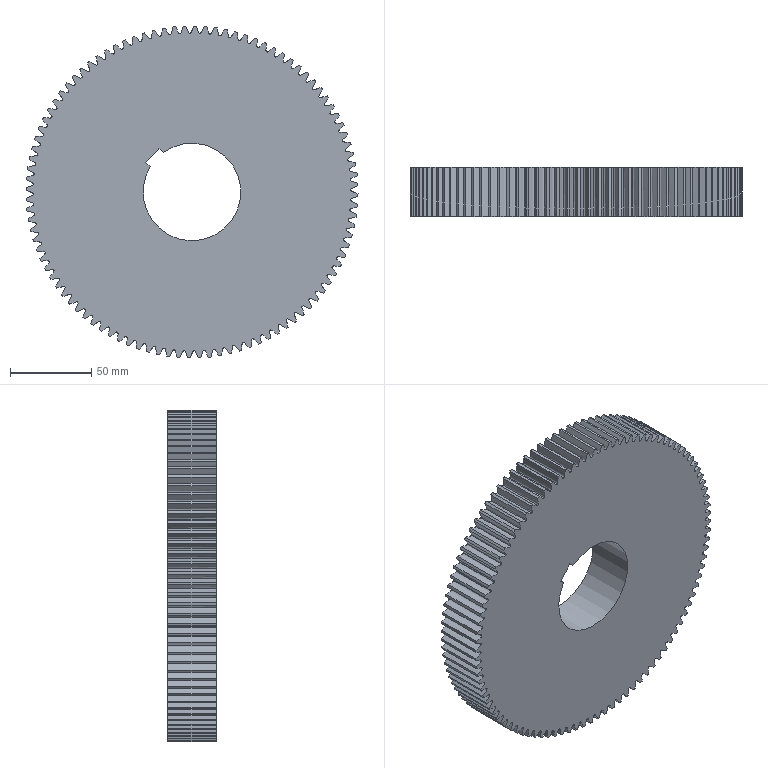Part | STEP file | 2026.6.15-Main Assembly图.sldasm-Part-33 | 1 solid | 408 faces | box 203.989 x 30 x 203.989 mm | volume 854746 mm3 | cylinder 203 | spline 200 | plane 5 | commonest cylinder face diameters 194.995 x100 204 x100 60 x3